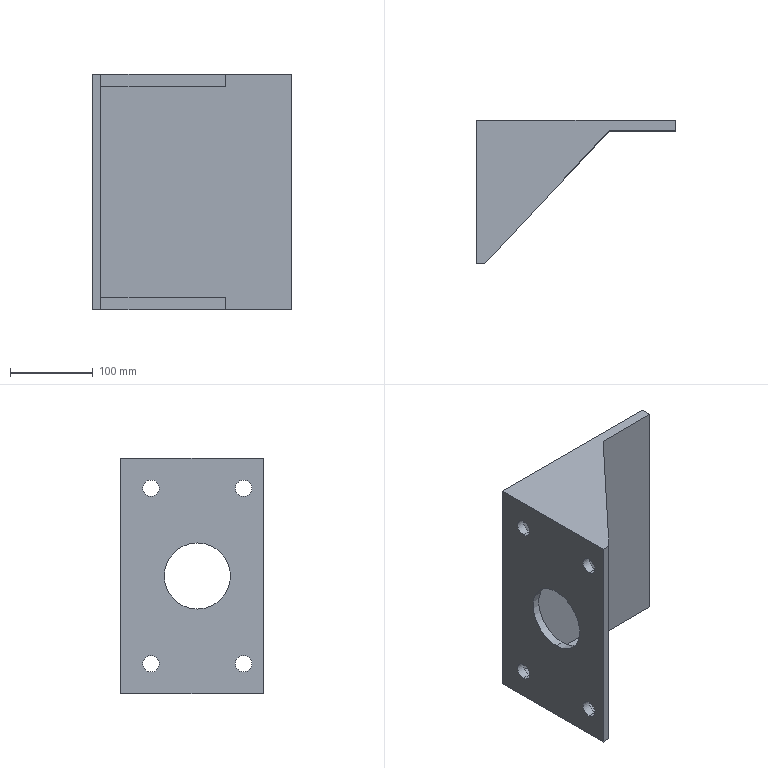Part | STEP file | Part 2 | 1 solid | 24 faces | box 240 x 172.72 x 285 mm | volume 1617851 mm3 | cylinder 12 | plane 12 | commonest cylinder face diameters 20 x8 21.34 x2 80 x2
STEP:
#1=CARTESIAN_POINT('',(36.903,-2.738,-127.5));
#2=VERTEX_POINT('',#1);
#3=CARTESIAN_POINT('',(36.903,-24.078,-127.5));
#4=VERTEX_POINT('',#3);
#5=CARTESIAN_POINT('',(36.903,-13.408,-127.5));
#6=DIRECTION('',(0.,0.,1.));
#7=DIRECTION('',(0.,-1.,0.));
#8=AXIS2_PLACEMENT_3D('',#5,#6,#7);
#9=CIRCLE('',#8,10.67);
#10=EDGE_CURVE('',#2,#4,#9,.T.);
#11=ORIENTED_EDGE('',*,*,#10,.T.);
#12=CARTESIAN_POINT('',(36.903,-24.078,-142.5));
#13=VERTEX_POINT('',#12);
#14=CARTESIAN_POINT('',(36.903,-24.078,-105.5));
#15=DIRECTION('',(0.,0.,-1.));
#16=VECTOR('',#15,1000.);
#17=LINE('',#14,#16);
#18=EDGE_CURVE('',#4,#13,#17,.T.);
#19=ORIENTED_EDGE('',*,*,#18,.T.);
#20=CARTESIAN_POINT('',(36.903,-2.738,-142.5));
#21=VERTEX_POINT('',#20);
#22=CARTESIAN_POINT('',(36.903,-13.408,-142.5));
#23=DIRECTION('',(0.,0.,-1.));
#24=DIRECTION('',(0.,1.,0.));
#25=AXIS2_PLACEMENT_3D('',#22,#23,#24);
#26=CIRCLE('',#25,10.67);
#27=EDGE_CURVE('',#13,#21,#26,.T.);
#28=ORIENTED_EDGE('',*,*,#27,.T.);
#29=CARTESIAN_POINT('',(36.903,-2.738,-105.5));
#30=DIRECTION('',(0.,0.,-1.));
#31=VECTOR('',#30,1000.);
#32=LINE('',#29,#31);
#33=EDGE_CURVE('',#2,#21,#32,.T.);
#34=ORIENTED_EDGE('',*,*,#33,.F.);
#35=EDGE_LOOP('',(#11,#19,#28,#34));
#36=FACE_OUTER_BOUND('',#35,.T.);
#37=CARTESIAN_POINT('',(36.903,-13.408,-105.5));
#38=DIRECTION('',(0.,0.,-1.));
#39=DIRECTION('',(0.,1.,0.));
#40=AXIS2_PLACEMENT_3D('',#37,#38,#39);
#41=CYLINDRICAL_SURFACE('',#40,10.67);
#42=ADVANCED_FACE('',(#36),#41,.F.);
#43=CARTESIAN_POINT('',(0.,0.,40.));
#44=VERTEX_POINT('',#43);
#45=CARTESIAN_POINT('',(0.,0.,-40.));
#46=VERTEX_POINT('',#45);
#47=CARTESIAN_POINT('',(0.,0.,0.));
#48=DIRECTION('',(1.,0.,0.));
#49=DIRECTION('',(0.,0.,-1.));
#50=AXIS2_PLACEMENT_3D('',#47,#48,#49);
#51=CIRCLE('',#50,40.);
#52=EDGE_CURVE('',#44,#46,#51,.T.);
#53=ORIENTED_EDGE('',*,*,#52,.F.);
#54=CARTESIAN_POINT('',(10.,0.,40.));
#55=VERTEX_POINT('',#54);
#56=CARTESIAN_POINT('',(0.,0.,40.));
#57=DIRECTION('',(1.,0.,0.));
#58=VECTOR('',#57,1000.);
#59=LINE('',#56,#58);
#60=EDGE_CURVE('',#44,#55,#59,.T.);
#61=ORIENTED_EDGE('',*,*,#60,.T.);
#62=CARTESIAN_POINT('',(10.,0.,-40.));
#63=VERTEX_POINT('',#62);
#64=CARTESIAN_POINT('',(10.,0.,0.));
#65=DIRECTION('',(1.,0.,0.));
#66=DIRECTION('',(0.,0.,-1.));
#67=AXIS2_PLACEMENT_3D('',#64,#65,#66);
#68=CIRCLE('',#67,40.);
#69=EDGE_CURVE('',#55,#63,#68,.T.);
#70=ORIENTED_EDGE('',*,*,#69,.T.);
#71=CARTESIAN_POINT('',(0.,0.,-40.));
#72=DIRECTION('',(1.,0.,0.));
#73=VECTOR('',#72,1000.);
#74=LINE('',#71,#73);
#75=EDGE_CURVE('',#46,#63,#74,.T.);
#76=ORIENTED_EDGE('',*,*,#75,.F.);
#77=EDGE_LOOP('',(#53,#61,#70,#76));
#78=FACE_OUTER_BOUND('',#77,.T.);
#79=CARTESIAN_POINT('',(0.,0.,0.));
#80=DIRECTION('',(1.,0.,0.));
#81=DIRECTION('',(0.,0.,-1.));
#82=AXIS2_PLACEMENT_3D('',#79,#80,#81);
#83=CYLINDRICAL_SURFACE('',#82,40.);
#84=ADVANCED_FACE('',(#78),#83,.F.);
#85=CARTESIAN_POINT('',(10.,-56.,-96.));
#86=VERTEX_POINT('',#85);
#87=CARTESIAN_POINT('',(10.,-56.,-116.));
#88=VERTEX_POINT('',#87);
#89=CARTESIAN_POINT('',(10.,-56.,-106.));
#90=DIRECTION('',(1.,0.,0.));
#91=DIRECTION('',(0.,0.,-1.));
#92=AXIS2_PLACEMENT_3D('',#89,#90,#91);
#93=CIRCLE('',#92,10.);
#94=EDGE_CURVE('',#86,#88,#93,.T.);
#95=ORIENTED_EDGE('',*,*,#94,.T.);
#96=CARTESIAN_POINT('',(0.,-56.,-116.));
#97=VERTEX_POINT('',#96);
#98=CARTESIAN_POINT('',(10.,-56.,-116.));
#99=DIRECTION('',(-1.,0.,0.));
#100=VECTOR('',#99,1000.);
#101=LINE('',#98,#100);
#102=EDGE_CURVE('',#88,#97,#101,.T.);
#103=ORIENTED_EDGE('',*,*,#102,.T.);
#104=CARTESIAN_POINT('',(0.,-56.,-96.));
#105=VERTEX_POINT('',#104);
#106=CARTESIAN_POINT('',(0.,-56.,-106.));
#107=DIRECTION('',(1.,0.,0.));
#108=DIRECTION('',(0.,0.,-1.));
#109=AXIS2_PLACEMENT_3D('',#106,#107,#108);
#110=CIRCLE('',#109,10.);
#111=EDGE_CURVE('',#105,#97,#110,.T.);
#112=ORIENTED_EDGE('',*,*,#111,.F.);
#113=CARTESIAN_POINT('',(10.,-56.,-96.));
#114=DIRECTION('',(-1.,0.,0.));
#115=VECTOR('',#114,1000.);
#116=LINE('',#113,#115);
#117=EDGE_CURVE('',#86,#105,#116,.T.);
#118=ORIENTED_EDGE('',*,*,#117,.F.);
#119=EDGE_LOOP('',(#95,#103,#112,#118));
#120=FACE_OUTER_BOUND('',#119,.T.);
#121=CARTESIAN_POINT('',(10.,-56.,-106.));
#122=DIRECTION('',(-1.,0.,0.));
#123=DIRECTION('',(0.,0.,1.));
#124=AXIS2_PLACEMENT_3D('',#121,#122,#123);
#125=CYLINDRICAL_SURFACE('',#124,10.);
#126=ADVANCED_FACE('',(#120),#125,.F.);
#127=CARTESIAN_POINT('',(10.,-56.,116.));
#128=VERTEX_POINT('',#127);
#129=CARTESIAN_POINT('',(10.,-56.,96.));
#130=VERTEX_POINT('',#129);
#131=CARTESIAN_POINT('',(10.,-56.,106.));
#132=DIRECTION('',(1.,0.,0.));
#133=DIRECTION('',(0.,0.,-1.));
#134=AXIS2_PLACEMENT_3D('',#131,#132,#133);
#135=CIRCLE('',#134,10.);
#136=EDGE_CURVE('',#128,#130,#135,.T.);
#137=ORIENTED_EDGE('',*,*,#136,.T.);
#138=CARTESIAN_POINT('',(0.,-56.,96.));
#139=VERTEX_POINT('',#138);
#140=CARTESIAN_POINT('',(10.,-56.,96.));
#141=DIRECTION('',(-1.,0.,0.));
#142=VECTOR('',#141,1000.);
#143=LINE('',#140,#142);
#144=EDGE_CURVE('',#130,#139,#143,.T.);
#145=ORIENTED_EDGE('',*,*,#144,.T.);
#146=CARTESIAN_POINT('',(0.,-56.,116.));
#147=VERTEX_POINT('',#146);
#148=CARTESIAN_POINT('',(0.,-56.,106.));
#149=DIRECTION('',(1.,0.,0.));
#150=DIRECTION('',(0.,0.,-1.));
#151=AXIS2_PLACEMENT_3D('',#148,#149,#150);
#152=CIRCLE('',#151,10.);
#153=EDGE_CURVE('',#147,#139,#152,.T.);
#154=ORIENTED_EDGE('',*,*,#153,.F.);
#155=CARTESIAN_POINT('',(10.,-56.,116.));
#156=DIRECTION('',(-1.,0.,0.));
#157=VECTOR('',#156,1000.);
#158=LINE('',#155,#157);
#159=EDGE_CURVE('',#128,#147,#158,.T.);
#160=ORIENTED_EDGE('',*,*,#159,.F.);
#161=EDGE_LOOP('',(#137,#145,#154,#160));
#162=FACE_OUTER_BOUND('',#161,.T.);
#163=CARTESIAN_POINT('',(10.,-56.,106.));
#164=DIRECTION('',(-1.,0.,0.));
#165=DIRECTION('',(0.,0.,1.));
#166=AXIS2_PLACEMENT_3D('',#163,#164,#165);
#167=CYLINDRICAL_SURFACE('',#166,10.);
#168=ADVANCED_FACE('',(#162),#167,.F.);
#169=CARTESIAN_POINT('',(10.,56.,-96.));
#170=VERTEX_POINT('',#169);
#171=CARTESIAN_POINT('',(10.,56.,-116.));
#172=VERTEX_POINT('',#171);
#173=CARTESIAN_POINT('',(10.,56.,-106.));
#174=DIRECTION('',(1.,0.,0.));
#175=DIRECTION('',(0.,0.,-1.));
#176=AXIS2_PLACEMENT_3D('',#173,#174,#175);
#177=CIRCLE('',#176,10.);
#178=EDGE_CURVE('',#170,#172,#177,.T.);
#179=ORIENTED_EDGE('',*,*,#178,.T.);
#180=CARTESIAN_POINT('',(0.,56.,-116.));
#181=VERTEX_POINT('',#180);
#182=CARTESIAN_POINT('',(10.,56.,-116.));
#183=DIRECTION('',(-1.,0.,0.));
#184=VECTOR('',#183,1000.);
#185=LINE('',#182,#184);
#186=EDGE_CURVE('',#172,#181,#185,.T.);
#187=ORIENTED_EDGE('',*,*,#186,.T.);
#188=CARTESIAN_POINT('',(0.,56.,-96.));
#189=VERTEX_POINT('',#188);
#190=CARTESIAN_POINT('',(0.,56.,-106.));
#191=DIRECTION('',(1.,0.,0.));
#192=DIRECTION('',(0.,0.,-1.));
#193=AXIS2_PLACEMENT_3D('',#190,#191,#192);
#194=CIRCLE('',#193,10.);
#195=EDGE_CURVE('',#189,#181,#194,.T.);
#196=ORIENTED_EDGE('',*,*,#195,.F.);
#197=CARTESIAN_POINT('',(10.,56.,-96.));
#198=DIRECTION('',(-1.,0.,0.));
#199=VECTOR('',#198,1000.);
#200=LINE('',#197,#199);
#201=EDGE_CURVE('',#170,#189,#200,.T.);
#202=ORIENTED_EDGE('',*,*,#201,.F.);
#203=EDGE_LOOP('',(#179,#187,#196,#202));
#204=FACE_OUTER_BOUND('',#203,.T.);
#205=CARTESIAN_POINT('',(10.,56.,-106.));
#206=DIRECTION('',(-1.,0.,0.));
#207=DIRECTION('',(0.,0.,1.));
#208=AXIS2_PLACEMENT_3D('',#205,#206,#207);
#209=CYLINDRICAL_SURFACE('',#208,10.);
#210=ADVANCED_FACE('',(#204),#209,.F.);
#211=CARTESIAN_POINT('',(10.,56.,116.));
#212=VERTEX_POINT('',#211);
#213=CARTESIAN_POINT('',(10.,56.,96.));
#214=VERTEX_POINT('',#213);
#215=CARTESIAN_POINT('',(10.,56.,106.));
#216=DIRECTION('',(1.,0.,0.));
#217=DIRECTION('',(0.,0.,-1.));
#218=AXIS2_PLACEMENT_3D('',#215,#216,#217);
#219=CIRCLE('',#218,10.);
#220=EDGE_CURVE('',#212,#214,#219,.T.);
#221=ORIENTED_EDGE('',*,*,#220,.T.);
#222=CARTESIAN_POINT('',(0.,56.,96.));
#223=VERTEX_POINT('',#222);
#224=CARTESIAN_POINT('',(10.,56.,96.));
#225=DIRECTION('',(-1.,0.,0.));
#226=VECTOR('',#225,1000.);
#227=LINE('',#224,#226);
#228=EDGE_CURVE('',#214,#223,#227,.T.);
#229=ORIENTED_EDGE('',*,*,#228,.T.);
#230=CARTESIAN_POINT('',(0.,56.,116.));
#231=VERTEX_POINT('',#230);
#232=CARTESIAN_POINT('',(0.,56.,106.));
#233=DIRECTION('',(1.,0.,0.));
#234=DIRECTION('',(0.,0.,-1.));
#235=AXIS2_PLACEMENT_3D('',#232,#233,#234);
#236=CIRCLE('',#235,10.);
#237=EDGE_CURVE('',#231,#223,#236,.T.);
#238=ORIENTED_EDGE('',*,*,#237,.F.);
#239=CARTESIAN_POINT('',(10.,56.,116.));
#240=DIRECTION('',(-1.,0.,0.));
#241=VECTOR('',#240,1000.);
#242=LINE('',#239,#241);
#243=EDGE_CURVE('',#212,#231,#242,.T.);
#244=ORIENTED_EDGE('',*,*,#243,.F.);
#245=EDGE_LOOP('',(#221,#229,#238,#244));
#246=FACE_OUTER_BOUND('',#245,.T.);
#247=CARTESIAN_POINT('',(10.,56.,106.));
#248=DIRECTION('',(-1.,0.,0.));
#249=DIRECTION('',(0.,0.,1.));
#250=AXIS2_PLACEMENT_3D('',#247,#248,#249);
#251=CYLINDRICAL_SURFACE('',#250,10.);
#252=ADVANCED_FACE('',(#246),#251,.F.);
#253=CARTESIAN_POINT('',(10.,0.,0.));
#254=DIRECTION('',(1.,0.,0.));
#255=DIRECTION('',(0.,0.,-1.));
#256=AXIS2_PLACEMENT_3D('',#253,#254,#255);
#257=CIRCLE('',#256,40.);
#258=EDGE_CURVE('',#63,#55,#257,.T.);
#259=ORIENTED_EDGE('',*,*,#258,.F.);
#260=ORIENTED_EDGE('',*,*,#69,.F.);
#261=EDGE_LOOP('',(#259,#260));
#262=FACE_BOUND('',#261,.T.);
#263=ORIENTED_EDGE('',*,*,#136,.F.);
#264=CARTESIAN_POINT('',(10.,-56.,106.));
#265=DIRECTION('',(1.,0.,0.));
#266=DIRECTION('',(0.,0.,-1.));
#267=AXIS2_PLACEMENT_3D('',#264,#265,#266);
#268=CIRCLE('',#267,10.);
#269=EDGE_CURVE('',#130,#128,#268,.T.);
#270=ORIENTED_EDGE('',*,*,#269,.F.);
#271=EDGE_LOOP('',(#263,#270));
#272=FACE_BOUND('',#271,.T.);
#273=ORIENTED_EDGE('',*,*,#220,.F.);
#274=CARTESIAN_POINT('',(10.,56.,106.));
#275=DIRECTION('',(1.,0.,0.));
#276=DIRECTION('',(0.,0.,-1.));
#277=AXIS2_PLACEMENT_3D('',#274,#275,#276);
#278=CIRCLE('',#277,10.);
#279=EDGE_CURVE('',#214,#212,#278,.T.);
#280=ORIENTED_EDGE('',*,*,#279,.F.);
#281=EDGE_LOOP('',(#273,#280));
#282=FACE_BOUND('',#281,.T.);
#283=ORIENTED_EDGE('',*,*,#178,.F.);
#284=CARTESIAN_POINT('',(10.,56.,-106.));
#285=DIRECTION('',(1.,0.,0.));
#286=DIRECTION('',(0.,0.,-1.));
#287=AXIS2_PLACEMENT_3D('',#284,#285,#286);
#288=CIRCLE('',#287,10.);
#289=EDGE_CURVE('',#172,#170,#288,.T.);
#290=ORIENTED_EDGE('',*,*,#289,.F.);
#291=EDGE_LOOP('',(#283,#290));
#292=FACE_BOUND('',#291,.T.);
#293=ORIENTED_EDGE('',*,*,#94,.F.);
#294=CARTESIAN_POINT('',(10.,-56.,-106.));
#295=DIRECTION('',(1.,0.,0.));
#296=DIRECTION('',(0.,0.,-1.));
#297=AXIS2_PLACEMENT_3D('',#294,#295,#296);
#298=CIRCLE('',#297,10.);
#299=EDGE_CURVE('',#88,#86,#298,.T.);
#300=ORIENTED_EDGE('',*,*,#299,.F.);
#301=EDGE_LOOP('',(#293,#300));
#302=FACE_BOUND('',#301,.T.);
#303=CARTESIAN_POINT('',(10.,80.,-127.5));
#304=VERTEX_POINT('',#303);
#305=CARTESIAN_POINT('',(10.,80.,127.5));
#306=VERTEX_POINT('',#305);
#307=CARTESIAN_POINT('',(10.,80.,127.5));
#308=DIRECTION('',(0.,0.,1.));
#309=VECTOR('',#308,1000.);
#310=LINE('',#307,#309);
#311=EDGE_CURVE('',#304,#306,#310,.T.);
#312=ORIENTED_EDGE('',*,*,#311,.T.);
#313=CARTESIAN_POINT('',(10.,-80.,127.5));
#314=VERTEX_POINT('',#313);
#315=CARTESIAN_POINT('',(10.,80.,127.5));
#316=DIRECTION('',(0.,-1.,0.));
#317=VECTOR('',#316,1000.);
#318=LINE('',#315,#317);
#319=EDGE_CURVE('',#306,#314,#318,.T.);
#320=ORIENTED_EDGE('',*,*,#319,.T.);
#321=CARTESIAN_POINT('',(10.,-80.,-127.5));
#322=VERTEX_POINT('',#321);
#323=CARTESIAN_POINT('',(10.,-80.,127.5));
#324=DIRECTION('',(0.,0.,-1.));
#325=VECTOR('',#324,1000.);
#326=LINE('',#323,#325);
#327=EDGE_CURVE('',#314,#322,#326,.T.);
#328=ORIENTED_EDGE('',*,*,#327,.T.);
#329=CARTESIAN_POINT('',(10.,0.,-127.5));
#330=DIRECTION('',(0.,-1.,0.));
#331=VECTOR('',#330,1000.);
#332=LINE('',#329,#331);
#333=EDGE_CURVE('',#304,#322,#332,.T.);
#334=ORIENTED_EDGE('',*,*,#333,.F.);
#335=EDGE_LOOP('',(#312,#320,#328,#334));
#336=FACE_OUTER_BOUND('',#335,.T.);
#337=CARTESIAN_POINT('',(10.,0.,0.));
#338=DIRECTION('',(1.,0.,0.));
#339=DIRECTION('',(0.,0.,-1.));
#340=AXIS2_PLACEMENT_3D('',#337,#338,#339);
#341=PLANE('',#340);
#342=ADVANCED_FACE('',(#262,#272,#282,#292,#302,#336),#341,.T.);
#343=CARTESIAN_POINT('',(0.,92.72,142.5));
#344=VERTEX_POINT('',#343);
#345=CARTESIAN_POINT('',(0.,92.72,-142.5));
#346=VERTEX_POINT('',#345);
#347=CARTESIAN_POINT('',(0.,92.72,-127.5));
#348=DIRECTION('',(0.,0.,-1.));
#349=VECTOR('',#348,1000.);
#350=LINE('',#347,#349);
#351=EDGE_CURVE('',#344,#346,#350,.T.);
#352=ORIENTED_EDGE('',*,*,#351,.T.);
#353=CARTESIAN_POINT('',(0.,-80.,-142.5));
#354=VERTEX_POINT('',#353);
#355=CARTESIAN_POINT('',(0.,-80.,-142.5));
#356=DIRECTION('',(0.,1.,0.));
#357=VECTOR('',#356,1000.);
#358=LINE('',#355,#357);
#359=EDGE_CURVE('',#354,#346,#358,.T.);
#360=ORIENTED_EDGE('',*,*,#359,.F.);
#361=CARTESIAN_POINT('',(0.,-80.,142.5));
#362=VERTEX_POINT('',#361);
#363=CARTESIAN_POINT('',(0.,-80.,127.5));
#364=DIRECTION('',(0.,0.,-1.));
#365=VECTOR('',#364,1000.);
#366=LINE('',#363,#365);
#367=EDGE_CURVE('',#362,#354,#366,.T.);
#368=ORIENTED_EDGE('',*,*,#367,.F.);
#369=CARTESIAN_POINT('',(0.,92.72,142.5));
#370=DIRECTION('',(0.,-1.,0.));
#371=VECTOR('',#370,1000.);
#372=LINE('',#369,#371);
#373=EDGE_CURVE('',#344,#362,#372,.T.);
#374=ORIENTED_EDGE('',*,*,#373,.F.);
#375=EDGE_LOOP('',(#352,#360,#368,#374));
#376=FACE_OUTER_BOUND('',#375,.T.);
#377=CARTESIAN_POINT('',(0.,0.,0.));
#378=DIRECTION('',(1.,0.,0.));
#379=DIRECTION('',(0.,0.,-1.));
#380=AXIS2_PLACEMENT_3D('',#377,#378,#379);
#381=CIRCLE('',#380,40.);
#382=EDGE_CURVE('',#46,#44,#381,.T.);
#383=ORIENTED_EDGE('',*,*,#382,.T.);
#384=ORIENTED_EDGE('',*,*,#52,.T.);
#385=EDGE_LOOP('',(#383,#384));
#386=FACE_BOUND('',#385,.T.);
#387=ORIENTED_EDGE('',*,*,#237,.T.);
#388=CARTESIAN_POINT('',(0.,56.,106.));
#389=DIRECTION('',(1.,0.,0.));
#390=DIRECTION('',(0.,0.,-1.));
#391=AXIS2_PLACEMENT_3D('',#388,#389,#390);
#392=CIRCLE('',#391,10.);
#393=EDGE_CURVE('',#223,#231,#392,.T.);
#394=ORIENTED_EDGE('',*,*,#393,.T.);
#395=EDGE_LOOP('',(#387,#394));
#396=FACE_BOUND('',#395,.T.);
#397=ORIENTED_EDGE('',*,*,#195,.T.);
#398=CARTESIAN_POINT('',(0.,56.,-106.));
#399=DIRECTION('',(1.,0.,0.));
#400=DIRECTION('',(0.,0.,-1.));
#401=AXIS2_PLACEMENT_3D('',#398,#399,#400);
#402=CIRCLE('',#401,10.);
#403=EDGE_CURVE('',#181,#189,#402,.T.);
#404=ORIENTED_EDGE('',*,*,#403,.T.);
#405=EDGE_LOOP('',(#397,#404));
#406=FACE_BOUND('',#405,.T.);
#407=ORIENTED_EDGE('',*,*,#153,.T.);
#408=CARTESIAN_POINT('',(0.,-56.,106.));
#409=DIRECTION('',(1.,0.,0.));
#410=DIRECTION('',(0.,0.,-1.));
#411=AXIS2_PLACEMENT_3D('',#408,#409,#410);
#412=CIRCLE('',#411,10.);
#413=EDGE_CURVE('',#139,#147,#412,.T.);
#414=ORIENTED_EDGE('',*,*,#413,.T.);
#415=EDGE_LOOP('',(#407,#414));
#416=FACE_BOUND('',#415,.T.);
#417=ORIENTED_EDGE('',*,*,#111,.T.);
#418=CARTESIAN_POINT('',(0.,-56.,-106.));
#419=DIRECTION('',(1.,0.,0.));
#420=DIRECTION('',(0.,0.,-1.));
#421=AXIS2_PLACEMENT_3D('',#418,#419,#420);
#422=CIRCLE('',#421,10.);
#423=EDGE_CURVE('',#97,#105,#422,.T.);
#424=ORIENTED_EDGE('',*,*,#423,.T.);
#425=EDGE_LOOP('',(#417,#424));
#426=FACE_BOUND('',#425,.T.);
#427=CARTESIAN_POINT('',(0.,0.,0.));
#428=DIRECTION('',(1.,0.,0.));
#429=DIRECTION('',(0.,0.,-1.));
#430=AXIS2_PLACEMENT_3D('',#427,#428,#429);
#431=PLANE('',#430);
#432=ADVANCED_FACE('',(#376,#386,#396,#406,#416,#426),#431,.F.);
#433=CARTESIAN_POINT('',(10.,-80.,-142.5));
#434=VERTEX_POINT('',#433);
#435=CARTESIAN_POINT('',(10.,-80.,-142.5));
#436=DIRECTION('',(-1.,0.,0.));
#437=VECTOR('',#436,1000.);
#438=LINE('',#435,#437);
#439=EDGE_CURVE('',#434,#354,#438,.T.);
#440=ORIENTED_EDGE('',*,*,#439,.F.);
#441=CARTESIAN_POINT('',(10.,-80.,-127.5));
#442=DIRECTION('',(0.,0.,-1.));
#443=VECTOR('',#442,1000.);
#444=LINE('',#441,#443);
#445=EDGE_CURVE('',#322,#434,#444,.T.);
#446=ORIENTED_EDGE('',*,*,#445,.F.);
#447=ORIENTED_EDGE('',*,*,#327,.F.);
#448=CARTESIAN_POINT('',(10.,-80.,142.5));
#449=VERTEX_POINT('',#448);
#450=CARTESIAN_POINT('',(10.,-80.,127.5));
#451=DIRECTION('',(0.,0.,-1.));
#452=VECTOR('',#451,1000.);
#453=LINE('',#450,#452);
#454=EDGE_CURVE('',#449,#314,#453,.T.);
#455=ORIENTED_EDGE('',*,*,#454,.F.);
#456=CARTESIAN_POINT('',(0.,-80.,142.5));
#457=DIRECTION('',(1.,0.,0.));
#458=VECTOR('',#457,1000.);
#459=LINE('',#456,#458);
#460=EDGE_CURVE('',#362,#449,#459,.T.);
#461=ORIENTED_EDGE('',*,*,#460,.F.);
#462=ORIENTED_EDGE('',*,*,#367,.T.);
#463=EDGE_LOOP('',(#440,#446,#447,#455,#461,#462));
#464=FACE_OUTER_BOUND('',#463,.T.);
#465=CARTESIAN_POINT('',(10.,-80.,127.5));
#466=DIRECTION('',(0.,1.,0.));
#467=DIRECTION('',(0.,0.,1.));
#468=AXIS2_PLACEMENT_3D('',#465,#466,#467);
#469=PLANE('',#468);
#470=ADVANCED_FACE('',(#464),#469,.F.);
#471=ORIENTED_EDGE('',*,*,#228,.F.);
#472=ORIENTED_EDGE('',*,*,#279,.T.);
#473=ORIENTED_EDGE('',*,*,#243,.T.);
#474=ORIENTED_EDGE('',*,*,#393,.F.);
#475=EDGE_LOOP('',(#471,#472,#473,#474));
#476=FACE_OUTER_BOUND('',#475,.T.);
#477=CARTESIAN_POINT('',(10.,56.,106.));
#478=DIRECTION('',(-1.,0.,0.));
#479=DIRECTION('',(0.,0.,1.));
#480=AXIS2_PLACEMENT_3D('',#477,#478,#479);
#481=CYLINDRICAL_SURFACE('',#480,10.);
#482=ADVANCED_FACE('',(#476),#481,.F.);
#483=ORIENTED_EDGE('',*,*,#186,.F.);
#484=ORIENTED_EDGE('',*,*,#289,.T.);
#485=ORIENTED_EDGE('',*,*,#201,.T.);
#486=ORIENTED_EDGE('',*,*,#403,.F.);
#487=EDGE_LOOP('',(#483,#484,#485,#486));
#488=FACE_OUTER_BOUND('',#487,.T.);
#489=CARTESIAN_POINT('',(10.,56.,-106.));
#490=DIRECTION('',(-1.,0.,0.));
#491=DIRECTION('',(0.,0.,1.));
#492=AXIS2_PLACEMENT_3D('',#489,#490,#491);
#493=CYLINDRICAL_SURFACE('',#492,10.);
#494=ADVANCED_FACE('',(#488),#493,.F.);
#495=ORIENTED_EDGE('',*,*,#144,.F.);
#496=ORIENTED_EDGE('',*,*,#269,.T.);
#497=ORIENTED_EDGE('',*,*,#159,.T.);
#498=ORIENTED_EDGE('',*,*,#413,.F.);
#499=EDGE_LOOP('',(#495,#496,#497,#498));
#500=FACE_OUTER_BOUND('',#499,.T.);
#501=CARTESIAN_POINT('',(10.,-56.,106.));
#502=DIRECTION('',(-1.,0.,0.));
#503=DIRECTION('',(0.,0.,1.));
#504=AXIS2_PLACEMENT_3D('',#501,#502,#503);
#505=CYLINDRICAL_SURFACE('',#504,10.);
#506=ADVANCED_FACE('',(#500),#505,.F.);
#507=ORIENTED_EDGE('',*,*,#102,.F.);
#508=ORIENTED_EDGE('',*,*,#299,.T.);
#509=ORIENTED_EDGE('',*,*,#117,.T.);
#510=ORIENTED_EDGE('',*,*,#423,.F.);
#511=EDGE_LOOP('',(#507,#508,#509,#510));
#512=FACE_OUTER_BOUND('',#511,.T.);
#513=CARTESIAN_POINT('',(10.,-56.,-106.));
#514=DIRECTION('',(-1.,0.,0.));
#515=DIRECTION('',(0.,0.,1.));
#516=AXIS2_PLACEMENT_3D('',#513,#514,#515);
#517=CYLINDRICAL_SURFACE('',#516,10.);
#518=ADVANCED_FACE('',(#512),#517,.F.);
#519=ORIENTED_EDGE('',*,*,#60,.F.);
#520=ORIENTED_EDGE('',*,*,#382,.F.);
#521=ORIENTED_EDGE('',*,*,#75,.T.);
#522=ORIENTED_EDGE('',*,*,#258,.T.);
#523=EDGE_LOOP('',(#519,#520,#521,#522));
#524=FACE_OUTER_BOUND('',#523,.T.);
#525=CARTESIAN_POINT('',(0.,0.,0.));
#526=DIRECTION('',(1.,0.,0.));
#527=DIRECTION('',(0.,0.,-1.));
#528=AXIS2_PLACEMENT_3D('',#525,#526,#527);
#529=CYLINDRICAL_SURFACE('',#528,40.);
#530=ADVANCED_FACE('',(#524),#529,.F.);
#531=CARTESIAN_POINT('',(160.,80.,127.5));
#532=VERTEX_POINT('',#531);
#533=CARTESIAN_POINT('',(160.,80.,142.5));
#534=VERTEX_POINT('',#533);
#535=CARTESIAN_POINT('',(160.,80.,127.5));
#536=DIRECTION('',(0.,0.,1.));
#537=VECTOR('',#536,1000.);
#538=LINE('',#535,#537);
#539=EDGE_CURVE('',#532,#534,#538,.T.);
#540=ORIENTED_EDGE('',*,*,#539,.F.);
#541=CARTESIAN_POINT('',(160.,80.,127.5));
#542=DIRECTION('',(-1.,0.,0.));
#543=VECTOR('',#542,1000.);
#544=LINE('',#541,#543);
#545=EDGE_CURVE('',#532,#306,#544,.T.);
#546=ORIENTED_EDGE('',*,*,#545,.T.);
#547=ORIENTED_EDGE('',*,*,#311,.F.);
#548=CARTESIAN_POINT('',(160.,80.,-127.5));
#549=VERTEX_POINT('',#548);
#550=CARTESIAN_POINT('',(240.,80.,-127.5));
#551=DIRECTION('',(-1.,0.,0.));
#552=VECTOR('',#551,1000.);
#553=LINE('',#550,#552);
#554=EDGE_CURVE('',#549,#304,#553,.T.);
#555=ORIENTED_EDGE('',*,*,#554,.F.);
#556=CARTESIAN_POINT('',(160.,80.,-142.5));
#557=VERTEX_POINT('',#556);
#558=CARTESIAN_POINT('',(160.,80.,-127.5));
#559=DIRECTION('',(0.,0.,-1.));
#560=VECTOR('',#559,1000.);
#561=LINE('',#558,#560);
#562=EDGE_CURVE('',#549,#557,#561,.T.);
#563=ORIENTED_EDGE('',*,*,#562,.T.);
#564=CARTESIAN_POINT('',(240.,80.,-142.5));
#565=VERTEX_POINT('',#564);
#566=CARTESIAN_POINT('',(240.,80.,-142.5));
#567=DIRECTION('',(-1.,0.,0.));
#568=VECTOR('',#567,1000.);
#569=LINE('',#566,#568);
#570=EDGE_CURVE('',#565,#557,#569,.T.);
#571=ORIENTED_EDGE('',*,*,#570,.F.);
#572=CARTESIAN_POINT('',(240.,80.,142.5));
#573=VERTEX_POINT('',#572);
#574=CARTESIAN_POINT('',(240.,80.,-127.5));
#575=DIRECTION('',(0.,0.,1.));
#576=VECTOR('',#575,1000.);
#577=LINE('',#574,#576);
#578=EDGE_CURVE('',#565,#573,#577,.T.);
#579=ORIENTED_EDGE('',*,*,#578,.T.);
#580=CARTESIAN_POINT('',(10.,80.,142.5));
#581=DIRECTION('',(1.,0.,0.));
#582=VECTOR('',#581,1000.);
#583=LINE('',#580,#582);
#584=EDGE_CURVE('',#534,#573,#583,.T.);
#585=ORIENTED_EDGE('',*,*,#584,.F.);
#586=EDGE_LOOP('',(#540,#546,#547,#555,#563,#571,#579,#585));
#587=FACE_OUTER_BOUND('',#586,.T.);
#588=CARTESIAN_POINT('',(240.,80.,-127.5));
#589=DIRECTION('',(0.,-1.,0.));
#590=DIRECTION('',(0.,0.,-1.));
#591=AXIS2_PLACEMENT_3D('',#588,#589,#590);
#592=PLANE('',#591);
#593=ADVANCED_FACE('',(#587),#592,.T.);
#594=CARTESIAN_POINT('',(240.,92.72,142.5));
#595=VERTEX_POINT('',#594);
#596=CARTESIAN_POINT('',(240.,92.72,-142.5));
#597=VERTEX_POINT('',#596);
#598=CARTESIAN_POINT('',(240.,92.72,-127.5));
#599=DIRECTION('',(0.,0.,-1.));
#600=VECTOR('',#599,1000.);
#601=LINE('',#598,#600);
#602=EDGE_CURVE('',#595,#597,#601,.T.);
#603=ORIENTED_EDGE('',*,*,#602,.T.);
#604=CARTESIAN_POINT('',(0.,92.72,-142.5));
#605=DIRECTION('',(1.,0.,0.));
#606=VECTOR('',#605,1000.);
#607=LINE('',#604,#606);
#608=EDGE_CURVE('',#346,#597,#607,.T.);
#609=ORIENTED_EDGE('',*,*,#608,.F.);
#610=ORIENTED_EDGE('',*,*,#351,.F.);
#611=CARTESIAN_POINT('',(240.,92.72,142.5));
#612=DIRECTION('',(-1.,0.,0.));
#613=VECTOR('',#612,1000.);
#614=LINE('',#611,#613);
#615=EDGE_CURVE('',#595,#344,#614,.T.);
#616=ORIENTED_EDGE('',*,*,#615,.F.);
#617=EDGE_LOOP('',(#603,#609,#610,#616));
#618=FACE_OUTER_BOUND('',#617,.T.);
#619=CARTESIAN_POINT('',(240.,92.72,-127.5));
#620=DIRECTION('',(0.,1.,0.));
#621=DIRECTION('',(0.,0.,1.));
#622=AXIS2_PLACEMENT_3D('',#619,#620,#621);
#623=PLANE('',#622);
#624=ADVANCED_FACE('',(#618),#623,.T.);
#625=CARTESIAN_POINT('',(240.,80.,142.5));
#626=DIRECTION('',(0.,1.,0.));
#627=VECTOR('',#626,1000.);
#628=LINE('',#625,#627);
#629=EDGE_CURVE('',#573,#595,#628,.T.);
#630=ORIENTED_EDGE('',*,*,#629,.F.);
#631=ORIENTED_EDGE('',*,*,#578,.F.);
#632=CARTESIAN_POINT('',(240.,92.72,-142.5));
#633=DIRECTION('',(0.,-1.,0.));
#634=VECTOR('',#633,1000.);
#635=LINE('',#632,#634);
#636=EDGE_CURVE('',#597,#565,#635,.T.);
#637=ORIENTED_EDGE('',*,*,#636,.F.);
#638=ORIENTED_EDGE('',*,*,#602,.F.);
#639=EDGE_LOOP('',(#630,#631,#637,#638));
#640=FACE_OUTER_BOUND('',#639,.T.);
#641=CARTESIAN_POINT('',(240.,0.,0.));
#642=DIRECTION('',(1.,0.,0.));
#643=DIRECTION('',(0.,0.,-1.));
#644=AXIS2_PLACEMENT_3D('',#641,#642,#643);
#645=PLANE('',#644);
#646=ADVANCED_FACE('',(#640),#645,.T.);
#647=CARTESIAN_POINT('',(36.903,-13.408,-142.5));
#648=DIRECTION('',(0.,0.,-1.));
#649=DIRECTION('',(0.,1.,0.));
#650=AXIS2_PLACEMENT_3D('',#647,#648,#649);
#651=CIRCLE('',#650,10.67);
#652=EDGE_CURVE('',#21,#13,#651,.T.);
#653=ORIENTED_EDGE('',*,*,#652,.F.);
#654=ORIENTED_EDGE('',*,*,#27,.F.);
#655=EDGE_LOOP('',(#653,#654));
#656=FACE_BOUND('',#655,.T.);
#657=CARTESIAN_POINT('',(160.,80.,-142.5));
#658=DIRECTION('',(-0.6839,-0.7295,0.));
#659=VECTOR('',#658,1000.);
#660=LINE('',#657,#659);
#661=EDGE_CURVE('',#557,#434,#660,.T.);
#662=ORIENTED_EDGE('',*,*,#661,.T.);
#663=ORIENTED_EDGE('',*,*,#439,.T.);
#664=ORIENTED_EDGE('',*,*,#359,.T.);
#665=ORIENTED_EDGE('',*,*,#608,.T.);
#666=ORIENTED_EDGE('',*,*,#636,.T.);
#667=ORIENTED_EDGE('',*,*,#570,.T.);
#668=EDGE_LOOP('',(#662,#663,#664,#665,#666,#667));
#669=FACE_OUTER_BOUND('',#668,.T.);
#670=CARTESIAN_POINT('',(0.,0.,-142.5));
#671=DIRECTION('',(0.,0.,-1.));
#672=DIRECTION('',(0.,1.,0.));
#673=AXIS2_PLACEMENT_3D('',#670,#671,#672);
#674=PLANE('',#673);
#675=ADVANCED_FACE('',(#656,#669),#674,.T.);
#676=ORIENTED_EDGE('',*,*,#460,.T.);
#677=CARTESIAN_POINT('',(10.,-80.,142.5));
#678=DIRECTION('',(0.6839,0.7295,0.));
#679=VECTOR('',#678,1000.);
#680=LINE('',#677,#679);
#681=EDGE_CURVE('',#449,#534,#680,.T.);
#682=ORIENTED_EDGE('',*,*,#681,.T.);
#683=ORIENTED_EDGE('',*,*,#584,.T.);
#684=ORIENTED_EDGE('',*,*,#629,.T.);
#685=ORIENTED_EDGE('',*,*,#615,.T.);
#686=ORIENTED_EDGE('',*,*,#373,.T.);
#687=EDGE_LOOP('',(#676,#682,#683,#684,#685,#686));
#688=FACE_OUTER_BOUND('',#687,.T.);
#689=CARTESIAN_POINT('',(0.,0.,142.5));
#690=DIRECTION('',(0.,0.,1.));
#691=DIRECTION('',(1.,0.,0.));
#692=AXIS2_PLACEMENT_3D('',#689,#690,#691);
#693=PLANE('',#692);
#694=ADVANCED_FACE('',(#688),#693,.T.);
#695=ORIENTED_EDGE('',*,*,#661,.F.);
#696=ORIENTED_EDGE('',*,*,#562,.F.);
#697=CARTESIAN_POINT('',(160.,80.,-127.5));
#698=DIRECTION('',(-0.6839,-0.7295,0.));
#699=VECTOR('',#698,1000.);
#700=LINE('',#697,#699);
#701=EDGE_CURVE('',#549,#322,#700,.T.);
#702=ORIENTED_EDGE('',*,*,#701,.T.);
#703=ORIENTED_EDGE('',*,*,#445,.T.);
#704=EDGE_LOOP('',(#695,#696,#702,#703));
#705=FACE_OUTER_BOUND('',#704,.T.);
#706=CARTESIAN_POINT('',(160.,80.,-127.5));
#707=DIRECTION('',(0.7295,-0.6839,0.));
#708=DIRECTION('',(0.6839,0.7295,0.));
#709=AXIS2_PLACEMENT_3D('',#706,#707,#708);
#710=PLANE('',#709);
#711=ADVANCED_FACE('',(#705),#710,.T.);
#712=ORIENTED_EDGE('',*,*,#10,.F.);
#713=CARTESIAN_POINT('',(36.903,-13.408,-127.5));
#714=DIRECTION('',(0.,0.,1.));
#715=DIRECTION('',(0.,-1.,0.));
#716=AXIS2_PLACEMENT_3D('',#713,#714,#715);
#717=CIRCLE('',#716,10.67);
#718=EDGE_CURVE('',#4,#2,#717,.T.);
#719=ORIENTED_EDGE('',*,*,#718,.F.);
#720=EDGE_LOOP('',(#712,#719));
#721=FACE_BOUND('',#720,.T.);
#722=ORIENTED_EDGE('',*,*,#554,.T.);
#723=ORIENTED_EDGE('',*,*,#333,.T.);
#724=ORIENTED_EDGE('',*,*,#701,.F.);
#725=EDGE_LOOP('',(#722,#723,#724));
#726=FACE_OUTER_BOUND('',#725,.T.);
#727=CARTESIAN_POINT('',(0.,0.,-127.5));
#728=DIRECTION('',(0.,0.,1.));
#729=DIRECTION('',(0.,-1.,0.));
#730=AXIS2_PLACEMENT_3D('',#727,#728,#729);
#731=PLANE('',#730);
#732=ADVANCED_FACE('',(#721,#726),#731,.T.);
#733=ORIENTED_EDGE('',*,*,#681,.F.);
#734=ORIENTED_EDGE('',*,*,#454,.T.);
#735=CARTESIAN_POINT('',(10.,-80.,127.5));
#736=DIRECTION('',(0.6839,0.7295,0.));
#737=VECTOR('',#736,1000.);
#738=LINE('',#735,#737);
#739=EDGE_CURVE('',#314,#532,#738,.T.);
#740=ORIENTED_EDGE('',*,*,#739,.T.);
#741=ORIENTED_EDGE('',*,*,#539,.T.);
#742=EDGE_LOOP('',(#733,#734,#740,#741));
#743=FACE_OUTER_BOUND('',#742,.T.);
#744=CARTESIAN_POINT('',(10.,-80.,127.5));
#745=DIRECTION('',(0.7295,-0.6839,0.));
#746=DIRECTION('',(0.6839,0.7295,0.));
#747=AXIS2_PLACEMENT_3D('',#744,#745,#746);
#748=PLANE('',#747);
#749=ADVANCED_FACE('',(#743),#748,.T.);
#750=ORIENTED_EDGE('',*,*,#739,.F.);
#751=ORIENTED_EDGE('',*,*,#319,.F.);
#752=ORIENTED_EDGE('',*,*,#545,.F.);
#753=EDGE_LOOP('',(#750,#751,#752));
#754=FACE_OUTER_BOUND('',#753,.T.);
#755=CARTESIAN_POINT('',(0.,0.,127.5));
#756=DIRECTION('',(0.,0.,1.));
#757=DIRECTION('',(1.,0.,0.));
#758=AXIS2_PLACEMENT_3D('',#755,#756,#757);
#759=PLANE('',#758);
#760=ADVANCED_FACE('',(#754),#759,.F.);
#761=ORIENTED_EDGE('',*,*,#18,.F.);
#762=ORIENTED_EDGE('',*,*,#718,.T.);
#763=ORIENTED_EDGE('',*,*,#33,.T.);
#764=ORIENTED_EDGE('',*,*,#652,.T.);
#765=EDGE_LOOP('',(#761,#762,#763,#764));
#766=FACE_OUTER_BOUND('',#765,.T.);
#767=CARTESIAN_POINT('',(36.903,-13.408,-105.5));
#768=DIRECTION('',(0.,0.,-1.));
#769=DIRECTION('',(0.,1.,0.));
#770=AXIS2_PLACEMENT_3D('',#767,#768,#769);
#771=CYLINDRICAL_SURFACE('',#770,10.67);
#772=ADVANCED_FACE('',(#766),#771,.F.);
#773=CLOSED_SHELL('',(#42,#84,#126,#168,#210,#252,#342,#432,#470,#482,#494,#506,#518,#530,#593,#624,#646,#675,#694,#711,#732,#749,#760,#772));
#774=MANIFOLD_SOLID_BREP('',#773);
#775=CARTESIAN_POINT('',(0.,0.,0.));
#776=DIRECTION('',(0.,0.,1.));
#777=DIRECTION('',(1.,0.,0.));
#778=AXIS2_PLACEMENT_3D('',#775,#776,#777);
#779=(LENGTH_UNIT()NAMED_UNIT(*)SI_UNIT(.MILLI.,.METRE.));
#780=UNCERTAINTY_MEASURE_WITH_UNIT(LENGTH_MEASURE(0.00001),#779,'','');
#781=(NAMED_UNIT(*)PLANE_ANGLE_UNIT()SI_UNIT($,.RADIAN.));
#782=(NAMED_UNIT(*)SI_UNIT($,.STERADIAN.)SOLID_ANGLE_UNIT());
#783=(GEOMETRIC_REPRESENTATION_CONTEXT(3)GLOBAL_UNCERTAINTY_ASSIGNED_CONTEXT((#780))GLOBAL_UNIT_ASSIGNED_CONTEXT((#779,#781,#782))REPRESENTATION_CONTEXT('',''));
#784=ADVANCED_BREP_SHAPE_REPRESENTATION('',(#774,#778),#783);